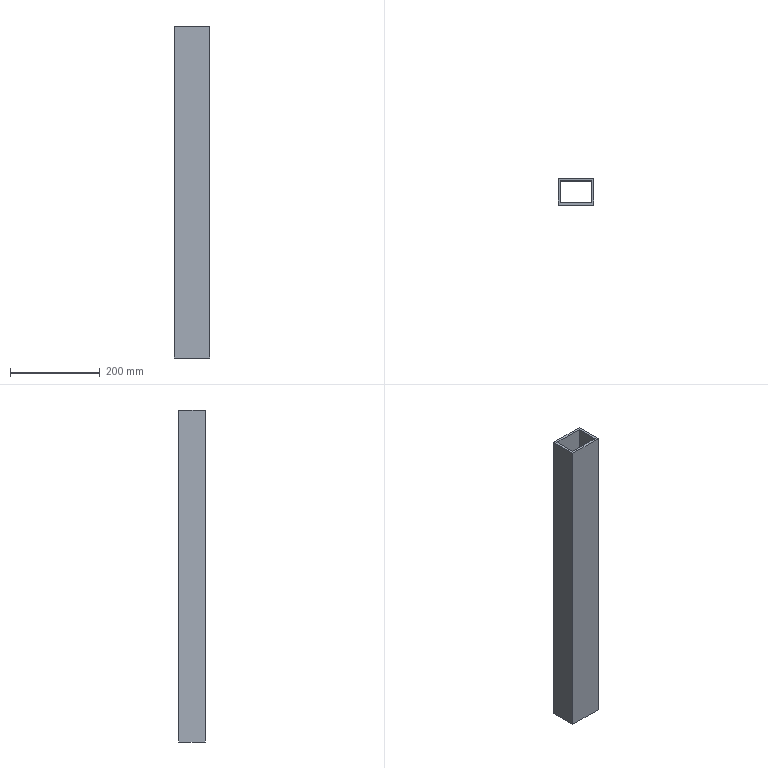Part | SolidWorks | features ICE 6, Cut 2, Extrusion 1 | 1 solid | 10 faces | box 80 x 60 x 740 mm | volume 962000 mm3 | plane 10
STEP:
#1=CARTESIAN_POINT('',(0.,-60.,740.));
#2=VERTEX_POINT('',#1);
#3=CARTESIAN_POINT('',(0.,-60.,0.));
#4=VERTEX_POINT('',#3);
#5=CARTESIAN_POINT('',(0.,-60.,740.));
#6=DIRECTION('',(0.,0.,-1.));
#7=VECTOR('',#6,1000.);
#8=LINE('',#5,#7);
#9=EDGE_CURVE('',#2,#4,#8,.T.);
#10=ORIENTED_EDGE('',*,*,#9,.F.);
#11=CARTESIAN_POINT('',(0.,0.,740.));
#12=VERTEX_POINT('',#11);
#13=CARTESIAN_POINT('',(0.,0.,740.));
#14=DIRECTION('',(0.,-1.,0.));
#15=VECTOR('',#14,1000.);
#16=LINE('',#13,#15);
#17=EDGE_CURVE('',#12,#2,#16,.T.);
#18=ORIENTED_EDGE('',*,*,#17,.F.);
#19=CARTESIAN_POINT('',(0.,0.,0.));
#20=VERTEX_POINT('',#19);
#21=CARTESIAN_POINT('',(0.,0.,740.));
#22=DIRECTION('',(0.,0.,-1.));
#23=VECTOR('',#22,1000.);
#24=LINE('',#21,#23);
#25=EDGE_CURVE('',#12,#20,#24,.T.);
#26=ORIENTED_EDGE('',*,*,#25,.T.);
#27=CARTESIAN_POINT('',(0.,-60.,0.));
#28=DIRECTION('',(0.,1.,0.));
#29=VECTOR('',#28,1000.);
#30=LINE('',#27,#29);
#31=EDGE_CURVE('',#4,#20,#30,.T.);
#32=ORIENTED_EDGE('',*,*,#31,.F.);
#33=EDGE_LOOP('',(#10,#18,#26,#32));
#34=FACE_OUTER_BOUND('',#33,.T.);
#35=CARTESIAN_POINT('',(0.,-60.,740.));
#36=DIRECTION('',(1.,0.,0.));
#37=DIRECTION('',(0.,0.,-1.));
#38=AXIS2_PLACEMENT_3D('',#35,#36,#37);
#39=PLANE('',#38);
#40=ADVANCED_FACE('',(#34),#39,.F.);
#41=ORIENTED_EDGE('',*,*,#9,.T.);
#42=CARTESIAN_POINT('',(80.,-60.,0.));
#43=VERTEX_POINT('',#42);
#44=CARTESIAN_POINT('',(80.,-60.,0.));
#45=DIRECTION('',(-1.,0.,0.));
#46=VECTOR('',#45,1000.);
#47=LINE('',#44,#46);
#48=EDGE_CURVE('',#43,#4,#47,.T.);
#49=ORIENTED_EDGE('',*,*,#48,.F.);
#50=CARTESIAN_POINT('',(80.,-60.,740.));
#51=VERTEX_POINT('',#50);
#52=CARTESIAN_POINT('',(80.,-60.,740.));
#53=DIRECTION('',(0.,0.,-1.));
#54=VECTOR('',#53,1000.);
#55=LINE('',#52,#54);
#56=EDGE_CURVE('',#51,#43,#55,.T.);
#57=ORIENTED_EDGE('',*,*,#56,.F.);
#58=CARTESIAN_POINT('',(0.,-60.,740.));
#59=DIRECTION('',(1.,0.,0.));
#60=VECTOR('',#59,1000.);
#61=LINE('',#58,#60);
#62=EDGE_CURVE('',#2,#51,#61,.T.);
#63=ORIENTED_EDGE('',*,*,#62,.F.);
#64=EDGE_LOOP('',(#41,#49,#57,#63));
#65=FACE_OUTER_BOUND('',#64,.T.);
#66=CARTESIAN_POINT('',(80.,-60.,740.));
#67=DIRECTION('',(0.,1.,0.));
#68=DIRECTION('',(0.,0.,1.));
#69=AXIS2_PLACEMENT_3D('',#66,#67,#68);
#70=PLANE('',#69);
#71=ADVANCED_FACE('',(#65),#70,.F.);
#72=CARTESIAN_POINT('',(80.,0.,740.));
#73=VERTEX_POINT('',#72);
#74=CARTESIAN_POINT('',(80.,-60.,740.));
#75=DIRECTION('',(0.,1.,0.));
#76=VECTOR('',#75,1000.);
#77=LINE('',#74,#76);
#78=EDGE_CURVE('',#51,#73,#77,.T.);
#79=ORIENTED_EDGE('',*,*,#78,.F.);
#80=ORIENTED_EDGE('',*,*,#56,.T.);
#81=CARTESIAN_POINT('',(80.,0.,0.));
#82=VERTEX_POINT('',#81);
#83=CARTESIAN_POINT('',(80.,0.,0.));
#84=DIRECTION('',(0.,-1.,0.));
#85=VECTOR('',#84,1000.);
#86=LINE('',#83,#85);
#87=EDGE_CURVE('',#82,#43,#86,.T.);
#88=ORIENTED_EDGE('',*,*,#87,.F.);
#89=CARTESIAN_POINT('',(80.,0.,740.));
#90=DIRECTION('',(0.,0.,-1.));
#91=VECTOR('',#90,1000.);
#92=LINE('',#89,#91);
#93=EDGE_CURVE('',#73,#82,#92,.T.);
#94=ORIENTED_EDGE('',*,*,#93,.F.);
#95=EDGE_LOOP('',(#79,#80,#88,#94));
#96=FACE_OUTER_BOUND('',#95,.T.);
#97=CARTESIAN_POINT('',(80.,0.,740.));
#98=DIRECTION('',(-1.,0.,0.));
#99=DIRECTION('',(0.,-1.,0.));
#100=AXIS2_PLACEMENT_3D('',#97,#98,#99);
#101=PLANE('',#100);
#102=ADVANCED_FACE('',(#96),#101,.F.);
#103=ORIENTED_EDGE('',*,*,#93,.T.);
#104=CARTESIAN_POINT('',(0.,0.,0.));
#105=DIRECTION('',(1.,0.,0.));
#106=VECTOR('',#105,1000.);
#107=LINE('',#104,#106);
#108=EDGE_CURVE('',#20,#82,#107,.T.);
#109=ORIENTED_EDGE('',*,*,#108,.F.);
#110=ORIENTED_EDGE('',*,*,#25,.F.);
#111=CARTESIAN_POINT('',(80.,0.,740.));
#112=DIRECTION('',(-1.,0.,0.));
#113=VECTOR('',#112,1000.);
#114=LINE('',#111,#113);
#115=EDGE_CURVE('',#73,#12,#114,.T.);
#116=ORIENTED_EDGE('',*,*,#115,.F.);
#117=EDGE_LOOP('',(#103,#109,#110,#116));
#118=FACE_OUTER_BOUND('',#117,.T.);
#119=CARTESIAN_POINT('',(0.,0.,740.));
#120=DIRECTION('',(0.,-1.,0.));
#121=DIRECTION('',(0.,0.,-1.));
#122=AXIS2_PLACEMENT_3D('',#119,#120,#121);
#123=PLANE('',#122);
#124=ADVANCED_FACE('',(#118),#123,.F.);
#125=ORIENTED_EDGE('',*,*,#17,.T.);
#126=ORIENTED_EDGE('',*,*,#62,.T.);
#127=ORIENTED_EDGE('',*,*,#78,.T.);
#128=ORIENTED_EDGE('',*,*,#115,.T.);
#129=EDGE_LOOP('',(#125,#126,#127,#128));
#130=FACE_OUTER_BOUND('',#129,.T.);
#131=CARTESIAN_POINT('',(75.,-5.,740.));
#132=VERTEX_POINT('',#131);
#133=CARTESIAN_POINT('',(75.,-55.,740.));
#134=VERTEX_POINT('',#133);
#135=CARTESIAN_POINT('',(75.,-5.,740.));
#136=DIRECTION('',(0.,-1.,0.));
#137=VECTOR('',#136,1000.);
#138=LINE('',#135,#137);
#139=EDGE_CURVE('',#132,#134,#138,.T.);
#140=ORIENTED_EDGE('',*,*,#139,.T.);
#141=CARTESIAN_POINT('',(5.,-55.,740.));
#142=VERTEX_POINT('',#141);
#143=CARTESIAN_POINT('',(5.,-55.,740.));
#144=DIRECTION('',(-1.,0.,0.));
#145=VECTOR('',#144,1000.);
#146=LINE('',#143,#145);
#147=EDGE_CURVE('',#134,#142,#146,.T.);
#148=ORIENTED_EDGE('',*,*,#147,.T.);
#149=CARTESIAN_POINT('',(5.,-5.,740.));
#150=VERTEX_POINT('',#149);
#151=CARTESIAN_POINT('',(5.,-55.,740.));
#152=DIRECTION('',(0.,1.,0.));
#153=VECTOR('',#152,1000.);
#154=LINE('',#151,#153);
#155=EDGE_CURVE('',#142,#150,#154,.T.);
#156=ORIENTED_EDGE('',*,*,#155,.T.);
#157=CARTESIAN_POINT('',(5.,-5.,740.));
#158=DIRECTION('',(1.,0.,0.));
#159=VECTOR('',#158,1000.);
#160=LINE('',#157,#159);
#161=EDGE_CURVE('',#150,#132,#160,.T.);
#162=ORIENTED_EDGE('',*,*,#161,.T.);
#163=EDGE_LOOP('',(#140,#148,#156,#162));
#164=FACE_BOUND('',#163,.T.);
#165=CARTESIAN_POINT('',(0.,0.,740.));
#166=DIRECTION('',(0.,0.,1.));
#167=DIRECTION('',(1.,0.,0.));
#168=AXIS2_PLACEMENT_3D('',#165,#166,#167);
#169=PLANE('',#168);
#170=ADVANCED_FACE('',(#130,#164),#169,.T.);
#171=ORIENTED_EDGE('',*,*,#48,.T.);
#172=ORIENTED_EDGE('',*,*,#31,.T.);
#173=ORIENTED_EDGE('',*,*,#108,.T.);
#174=ORIENTED_EDGE('',*,*,#87,.T.);
#175=EDGE_LOOP('',(#171,#172,#173,#174));
#176=FACE_OUTER_BOUND('',#175,.T.);
#177=CARTESIAN_POINT('',(75.,-55.,0.));
#178=VERTEX_POINT('',#177);
#179=CARTESIAN_POINT('',(5.,-55.,0.));
#180=VERTEX_POINT('',#179);
#181=CARTESIAN_POINT('',(5.,-55.,0.));
#182=DIRECTION('',(-1.,0.,0.));
#183=VECTOR('',#182,1000.);
#184=LINE('',#181,#183);
#185=EDGE_CURVE('',#178,#180,#184,.T.);
#186=ORIENTED_EDGE('',*,*,#185,.F.);
#187=CARTESIAN_POINT('',(75.,-5.,0.));
#188=VERTEX_POINT('',#187);
#189=CARTESIAN_POINT('',(75.,-5.,0.));
#190=DIRECTION('',(0.,-1.,0.));
#191=VECTOR('',#190,1000.);
#192=LINE('',#189,#191);
#193=EDGE_CURVE('',#188,#178,#192,.T.);
#194=ORIENTED_EDGE('',*,*,#193,.F.);
#195=CARTESIAN_POINT('',(5.,-5.,0.));
#196=VERTEX_POINT('',#195);
#197=CARTESIAN_POINT('',(5.,-5.,0.));
#198=DIRECTION('',(1.,0.,0.));
#199=VECTOR('',#198,1000.);
#200=LINE('',#197,#199);
#201=EDGE_CURVE('',#196,#188,#200,.T.);
#202=ORIENTED_EDGE('',*,*,#201,.F.);
#203=CARTESIAN_POINT('',(5.,-55.,0.));
#204=DIRECTION('',(0.,1.,0.));
#205=VECTOR('',#204,1000.);
#206=LINE('',#203,#205);
#207=EDGE_CURVE('',#180,#196,#206,.T.);
#208=ORIENTED_EDGE('',*,*,#207,.F.);
#209=EDGE_LOOP('',(#186,#194,#202,#208));
#210=FACE_BOUND('',#209,.T.);
#211=CARTESIAN_POINT('',(0.,0.,0.));
#212=DIRECTION('',(0.,0.,-1.));
#213=DIRECTION('',(-1.,0.,0.));
#214=AXIS2_PLACEMENT_3D('',#211,#212,#213);
#215=PLANE('',#214);
#216=ADVANCED_FACE('',(#176,#210),#215,.T.);
#217=ORIENTED_EDGE('',*,*,#185,.T.);
#218=CARTESIAN_POINT('',(5.,-55.,740.));
#219=DIRECTION('',(0.,0.,-1.));
#220=VECTOR('',#219,1000.);
#221=LINE('',#218,#220);
#222=EDGE_CURVE('',#142,#180,#221,.T.);
#223=ORIENTED_EDGE('',*,*,#222,.F.);
#224=ORIENTED_EDGE('',*,*,#147,.F.);
#225=CARTESIAN_POINT('',(75.,-55.,740.));
#226=DIRECTION('',(0.,0.,-1.));
#227=VECTOR('',#226,1000.);
#228=LINE('',#225,#227);
#229=EDGE_CURVE('',#134,#178,#228,.T.);
#230=ORIENTED_EDGE('',*,*,#229,.T.);
#231=EDGE_LOOP('',(#217,#223,#224,#230));
#232=FACE_OUTER_BOUND('',#231,.T.);
#233=CARTESIAN_POINT('',(5.,-55.,740.));
#234=DIRECTION('',(0.,-1.,0.));
#235=DIRECTION('',(0.,0.,-1.));
#236=AXIS2_PLACEMENT_3D('',#233,#234,#235);
#237=PLANE('',#236);
#238=ADVANCED_FACE('',(#232),#237,.F.);
#239=ORIENTED_EDGE('',*,*,#193,.T.);
#240=ORIENTED_EDGE('',*,*,#229,.F.);
#241=ORIENTED_EDGE('',*,*,#139,.F.);
#242=CARTESIAN_POINT('',(75.,-5.,740.));
#243=DIRECTION('',(0.,0.,-1.));
#244=VECTOR('',#243,1000.);
#245=LINE('',#242,#244);
#246=EDGE_CURVE('',#132,#188,#245,.T.);
#247=ORIENTED_EDGE('',*,*,#246,.T.);
#248=EDGE_LOOP('',(#239,#240,#241,#247));
#249=FACE_OUTER_BOUND('',#248,.T.);
#250=CARTESIAN_POINT('',(75.,-5.,740.));
#251=DIRECTION('',(1.,0.,0.));
#252=DIRECTION('',(0.,0.,-1.));
#253=AXIS2_PLACEMENT_3D('',#250,#251,#252);
#254=PLANE('',#253);
#255=ADVANCED_FACE('',(#249),#254,.F.);
#256=ORIENTED_EDGE('',*,*,#201,.T.);
#257=ORIENTED_EDGE('',*,*,#246,.F.);
#258=ORIENTED_EDGE('',*,*,#161,.F.);
#259=CARTESIAN_POINT('',(5.,-5.,740.));
#260=DIRECTION('',(0.,0.,-1.));
#261=VECTOR('',#260,1000.);
#262=LINE('',#259,#261);
#263=EDGE_CURVE('',#150,#196,#262,.T.);
#264=ORIENTED_EDGE('',*,*,#263,.T.);
#265=EDGE_LOOP('',(#256,#257,#258,#264));
#266=FACE_OUTER_BOUND('',#265,.T.);
#267=CARTESIAN_POINT('',(5.,-5.,740.));
#268=DIRECTION('',(0.,1.,0.));
#269=DIRECTION('',(0.,0.,1.));
#270=AXIS2_PLACEMENT_3D('',#267,#268,#269);
#271=PLANE('',#270);
#272=ADVANCED_FACE('',(#266),#271,.F.);
#273=ORIENTED_EDGE('',*,*,#207,.T.);
#274=ORIENTED_EDGE('',*,*,#263,.F.);
#275=ORIENTED_EDGE('',*,*,#155,.F.);
#276=ORIENTED_EDGE('',*,*,#222,.T.);
#277=EDGE_LOOP('',(#273,#274,#275,#276));
#278=FACE_OUTER_BOUND('',#277,.T.);
#279=CARTESIAN_POINT('',(5.,-55.,740.));
#280=DIRECTION('',(-1.,0.,0.));
#281=DIRECTION('',(0.,0.,1.));
#282=AXIS2_PLACEMENT_3D('',#279,#280,#281);
#283=PLANE('',#282);
#284=ADVANCED_FACE('',(#278),#283,.F.);
#285=CLOSED_SHELL('',(#40,#71,#102,#124,#170,#216,#238,#255,#272,#284));
#286=MANIFOLD_SOLID_BREP('',#285);
#287=CARTESIAN_POINT('',(0.,0.,0.));
#288=DIRECTION('',(0.,0.,1.));
#289=DIRECTION('',(1.,0.,0.));
#290=AXIS2_PLACEMENT_3D('',#287,#288,#289);
#291=(LENGTH_UNIT()NAMED_UNIT(*)SI_UNIT(.MILLI.,.METRE.));
#292=UNCERTAINTY_MEASURE_WITH_UNIT(LENGTH_MEASURE(0.00001),#291,'','');
#293=(NAMED_UNIT(*)PLANE_ANGLE_UNIT()SI_UNIT($,.RADIAN.));
#294=(NAMED_UNIT(*)SI_UNIT($,.STERADIAN.)SOLID_ANGLE_UNIT());
#295=(GEOMETRIC_REPRESENTATION_CONTEXT(3)GLOBAL_UNCERTAINTY_ASSIGNED_CONTEXT((#292))GLOBAL_UNIT_ASSIGNED_CONTEXT((#291,#293,#294))REPRESENTATION_CONTEXT('',''));
#296=ADVANCED_BREP_SHAPE_REPRESENTATION('',(#286,#290),#295);